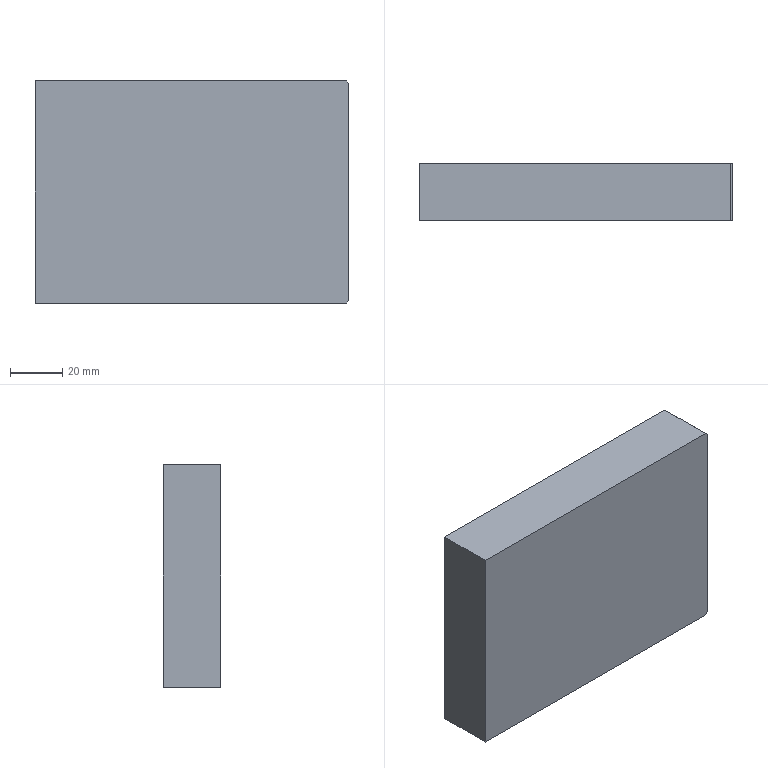Part | STEP file | B1-023 | 1 solid | 8 faces | box 120 x 22 x 85 mm | volume 224378 mm3 | plane 8
STEP:
#1=CARTESIAN_POINT('',(0.,0.,0.));
#2=DIRECTION('',(0.,0.,1.));
#3=DIRECTION('',(1.,0.,0.));
#4=AXIS2_PLACEMENT_3D('',#1,#2,#3);
#5=CARTESIAN_POINT('',(59.,11.,-42.5));
#6=VERTEX_POINT('',#5);
#7=CARTESIAN_POINT('',(-60.,11.,-42.5));
#8=VERTEX_POINT('',#7);
#9=CARTESIAN_POINT('',(60.,11.,-42.5));
#10=DIRECTION('',(-1.,0.,0.));
#11=VECTOR('',#10,1.);
#12=LINE('',#9,#11);
#13=CARTESIAN_POINT('',(60.,11.,-42.5));
#14=DIRECTION('',(0.,0.,1.));
#15=DIRECTION('',(1.,0.,0.));
#16=AXIS2_PLACEMENT_3D('',#13,#14,#15);
#17=PLANE('',#16);
#18=CARTESIAN_POINT('',(0.,0.));
#19=DIRECTION('',(-1.,0.));
#20=VECTOR('',#19,1.);
#21=LINE('',#18,#20);
#22=(GEOMETRIC_REPRESENTATION_CONTEXT(2)PARAMETRIC_REPRESENTATION_CONTEXT()REPRESENTATION_CONTEXT('',''));
#23=DEFINITIONAL_REPRESENTATION('',(#21),#22);
#24=PCURVE('',#17,#23);
#25=CARTESIAN_POINT('',(60.,11.,42.5));
#26=DIRECTION('',(0.,-1.,0.));
#27=DIRECTION('',(0.,0.,-1.));
#28=AXIS2_PLACEMENT_3D('',#25,#26,#27);
#29=PLANE('',#28);
#30=CARTESIAN_POINT('',(85.,0.));
#31=DIRECTION('',(0.,-1.));
#32=VECTOR('',#31,1.);
#33=LINE('',#30,#32);
#34=(GEOMETRIC_REPRESENTATION_CONTEXT(2)PARAMETRIC_REPRESENTATION_CONTEXT()REPRESENTATION_CONTEXT('',''));
#35=DEFINITIONAL_REPRESENTATION('',(#33),#34);
#36=PCURVE('',#29,#35);
#37=SURFACE_CURVE('',#12,(#24,#36),.PCURVE_S1.);
#38=EDGE_CURVE('',#6,#8,#37,.T.);
#39=ORIENTED_EDGE('',*,*,#38,.F.);
#40=CARTESIAN_POINT('',(59.,-11.,-42.5));
#41=VERTEX_POINT('',#40);
#42=CARTESIAN_POINT('',(59.,-11.,-42.5));
#43=DIRECTION('',(0.,-1.,0.));
#44=VECTOR('',#43,1.);
#45=LINE('',#42,#44);
#46=CARTESIAN_POINT('',(-1.,-22.));
#47=DIRECTION('',(0.,-1.));
#48=VECTOR('',#47,1.);
#49=LINE('',#46,#48);
#50=(GEOMETRIC_REPRESENTATION_CONTEXT(2)PARAMETRIC_REPRESENTATION_CONTEXT()REPRESENTATION_CONTEXT('',''));
#51=DEFINITIONAL_REPRESENTATION('',(#49),#50);
#52=PCURVE('',#17,#51);
#53=CARTESIAN_POINT('',(60.,0.,-41.5));
#54=DIRECTION('',(0.7071,0.,-0.7071));
#55=DIRECTION('',(0.,-1.,0.));
#56=AXIS2_PLACEMENT_3D('',#53,#54,#55);
#57=PLANE('',#56);
#58=CARTESIAN_POINT('',(11.,1.414));
#59=DIRECTION('',(1.,0.));
#60=VECTOR('',#59,1.);
#61=LINE('',#58,#60);
#62=(GEOMETRIC_REPRESENTATION_CONTEXT(2)PARAMETRIC_REPRESENTATION_CONTEXT()REPRESENTATION_CONTEXT('',''));
#63=DEFINITIONAL_REPRESENTATION('',(#61),#62);
#64=PCURVE('',#57,#63);
#65=SURFACE_CURVE('',#45,(#52,#64),.PCURVE_S1.);
#66=EDGE_CURVE('',#6,#41,#65,.T.);
#67=ORIENTED_EDGE('',*,*,#66,.T.);
#68=CARTESIAN_POINT('',(-60.,-11.,-42.5));
#69=VERTEX_POINT('',#68);
#70=CARTESIAN_POINT('',(60.,-11.,-42.5));
#71=DIRECTION('',(-1.,0.,0.));
#72=VECTOR('',#71,1.);
#73=LINE('',#70,#72);
#74=CARTESIAN_POINT('',(0.,-22.));
#75=DIRECTION('',(-1.,0.));
#76=VECTOR('',#75,1.);
#77=LINE('',#74,#76);
#78=(GEOMETRIC_REPRESENTATION_CONTEXT(2)PARAMETRIC_REPRESENTATION_CONTEXT()REPRESENTATION_CONTEXT('',''));
#79=DEFINITIONAL_REPRESENTATION('',(#77),#78);
#80=PCURVE('',#17,#79);
#81=CARTESIAN_POINT('',(60.,-11.,42.5));
#82=DIRECTION('',(0.,1.,0.));
#83=DIRECTION('',(0.,0.,1.));
#84=AXIS2_PLACEMENT_3D('',#81,#82,#83);
#85=PLANE('',#84);
#86=CARTESIAN_POINT('',(-85.,0.));
#87=DIRECTION('',(0.,-1.));
#88=VECTOR('',#87,1.);
#89=LINE('',#86,#88);
#90=(GEOMETRIC_REPRESENTATION_CONTEXT(2)PARAMETRIC_REPRESENTATION_CONTEXT()REPRESENTATION_CONTEXT('',''));
#91=DEFINITIONAL_REPRESENTATION('',(#89),#90);
#92=PCURVE('',#85,#91);
#93=SURFACE_CURVE('',#73,(#80,#92),.PCURVE_S1.);
#94=EDGE_CURVE('',#41,#69,#93,.T.);
#95=ORIENTED_EDGE('',*,*,#94,.T.);
#96=CARTESIAN_POINT('',(-60.,11.,-42.5));
#97=DIRECTION('',(0.,1.,0.));
#98=VECTOR('',#97,1.);
#99=LINE('',#96,#98);
#100=CARTESIAN_POINT('',(-120.,0.));
#101=DIRECTION('',(0.,1.));
#102=VECTOR('',#101,1.);
#103=LINE('',#100,#102);
#104=(GEOMETRIC_REPRESENTATION_CONTEXT(2)PARAMETRIC_REPRESENTATION_CONTEXT()REPRESENTATION_CONTEXT('',''));
#105=DEFINITIONAL_REPRESENTATION('',(#103),#104);
#106=PCURVE('',#17,#105);
#107=CARTESIAN_POINT('',(-60.,0.,0.));
#108=DIRECTION('',(1.,0.,0.));
#109=DIRECTION('',(0.,0.,-1.));
#110=AXIS2_PLACEMENT_3D('',#107,#108,#109);
#111=PLANE('',#110);
#112=CARTESIAN_POINT('',(42.5,11.));
#113=DIRECTION('',(0.,1.));
#114=VECTOR('',#113,1.);
#115=LINE('',#112,#114);
#116=(GEOMETRIC_REPRESENTATION_CONTEXT(2)PARAMETRIC_REPRESENTATION_CONTEXT()REPRESENTATION_CONTEXT('',''));
#117=DEFINITIONAL_REPRESENTATION('',(#115),#116);
#118=PCURVE('',#111,#117);
#119=SURFACE_CURVE('',#99,(#106,#118),.PCURVE_S1.);
#120=EDGE_CURVE('',#69,#8,#119,.T.);
#121=ORIENTED_EDGE('',*,*,#120,.T.);
#122=EDGE_LOOP('',(#39,#67,#95,#121));
#123=FACE_BOUND('',#122,.T.);
#124=ADVANCED_FACE('',(#123),#17,.F.);
#125=CARTESIAN_POINT('',(59.,11.,42.5));
#126=VERTEX_POINT('',#125);
#127=CARTESIAN_POINT('',(-60.,11.,42.5));
#128=VERTEX_POINT('',#127);
#129=CARTESIAN_POINT('',(60.,11.,42.5));
#130=DIRECTION('',(-1.,0.,0.));
#131=VECTOR('',#130,1.);
#132=LINE('',#129,#131);
#133=CARTESIAN_POINT('',(0.,0.));
#134=DIRECTION('',(0.,-1.));
#135=VECTOR('',#134,1.);
#136=LINE('',#133,#135);
#137=(GEOMETRIC_REPRESENTATION_CONTEXT(2)PARAMETRIC_REPRESENTATION_CONTEXT()REPRESENTATION_CONTEXT('',''));
#138=DEFINITIONAL_REPRESENTATION('',(#136),#137);
#139=PCURVE('',#29,#138);
#140=CARTESIAN_POINT('',(60.,11.,42.5));
#141=DIRECTION('',(0.,0.,-1.));
#142=DIRECTION('',(-1.,0.,0.));
#143=AXIS2_PLACEMENT_3D('',#140,#141,#142);
#144=PLANE('',#143);
#145=CARTESIAN_POINT('',(0.,0.));
#146=DIRECTION('',(1.,0.));
#147=VECTOR('',#146,1.);
#148=LINE('',#145,#147);
#149=(GEOMETRIC_REPRESENTATION_CONTEXT(2)PARAMETRIC_REPRESENTATION_CONTEXT()REPRESENTATION_CONTEXT('',''));
#150=DEFINITIONAL_REPRESENTATION('',(#148),#149);
#151=PCURVE('',#144,#150);
#152=SURFACE_CURVE('',#132,(#139,#151),.PCURVE_S1.);
#153=EDGE_CURVE('',#126,#128,#152,.T.);
#154=ORIENTED_EDGE('',*,*,#153,.F.);
#155=CARTESIAN_POINT('',(60.,11.,41.5));
#156=VERTEX_POINT('',#155);
#157=CARTESIAN_POINT('',(60.,11.,41.5));
#158=DIRECTION('',(0.7071,0.,-0.7071));
#159=VECTOR('',#158,1.);
#160=LINE('',#157,#159);
#161=CARTESIAN_POINT('',(1.,0.));
#162=DIRECTION('',(0.7071,0.7071));
#163=VECTOR('',#162,1.);
#164=LINE('',#161,#163);
#165=(GEOMETRIC_REPRESENTATION_CONTEXT(2)PARAMETRIC_REPRESENTATION_CONTEXT()REPRESENTATION_CONTEXT('',''));
#166=DEFINITIONAL_REPRESENTATION('',(#164),#165);
#167=PCURVE('',#29,#166);
#168=CARTESIAN_POINT('',(60.,0.,41.5));
#169=DIRECTION('',(0.7071,0.,0.7071));
#170=DIRECTION('',(0.,1.,0.));
#171=AXIS2_PLACEMENT_3D('',#168,#169,#170);
#172=PLANE('',#171);
#173=CARTESIAN_POINT('',(11.,0.));
#174=DIRECTION('',(0.,-1.));
#175=VECTOR('',#174,1.);
#176=LINE('',#173,#175);
#177=(GEOMETRIC_REPRESENTATION_CONTEXT(2)PARAMETRIC_REPRESENTATION_CONTEXT()REPRESENTATION_CONTEXT('',''));
#178=DEFINITIONAL_REPRESENTATION('',(#176),#177);
#179=PCURVE('',#172,#178);
#180=SURFACE_CURVE('',#160,(#167,#179),.PCURVE_S1.);
#181=EDGE_CURVE('',#126,#156,#180,.T.);
#182=ORIENTED_EDGE('',*,*,#181,.T.);
#183=CARTESIAN_POINT('',(60.,11.,-41.5));
#184=VERTEX_POINT('',#183);
#185=CARTESIAN_POINT('',(60.,11.,42.5));
#186=DIRECTION('',(0.,0.,1.));
#187=VECTOR('',#186,1.);
#188=LINE('',#185,#187);
#189=CARTESIAN_POINT('',(0.,0.));
#190=DIRECTION('',(-1.,0.));
#191=VECTOR('',#190,1.);
#192=LINE('',#189,#191);
#193=(GEOMETRIC_REPRESENTATION_CONTEXT(2)PARAMETRIC_REPRESENTATION_CONTEXT()REPRESENTATION_CONTEXT('',''));
#194=DEFINITIONAL_REPRESENTATION('',(#192),#193);
#195=PCURVE('',#29,#194);
#196=CARTESIAN_POINT('',(60.,0.,0.));
#197=DIRECTION('',(1.,0.,0.));
#198=DIRECTION('',(0.,0.,-1.));
#199=AXIS2_PLACEMENT_3D('',#196,#197,#198);
#200=PLANE('',#199);
#201=CARTESIAN_POINT('',(-42.5,11.));
#202=DIRECTION('',(-1.,0.));
#203=VECTOR('',#202,1.);
#204=LINE('',#201,#203);
#205=(GEOMETRIC_REPRESENTATION_CONTEXT(2)PARAMETRIC_REPRESENTATION_CONTEXT()REPRESENTATION_CONTEXT('',''));
#206=DEFINITIONAL_REPRESENTATION('',(#204),#205);
#207=PCURVE('',#200,#206);
#208=SURFACE_CURVE('',#188,(#195,#207),.PCURVE_S1.);
#209=EDGE_CURVE('',#184,#156,#208,.T.);
#210=ORIENTED_EDGE('',*,*,#209,.F.);
#211=CARTESIAN_POINT('',(60.,11.,-41.5));
#212=DIRECTION('',(-0.7071,0.,-0.7071));
#213=VECTOR('',#212,1.);
#214=LINE('',#211,#213);
#215=CARTESIAN_POINT('',(84.,0.));
#216=DIRECTION('',(0.7071,-0.7071));
#217=VECTOR('',#216,1.);
#218=LINE('',#215,#217);
#219=(GEOMETRIC_REPRESENTATION_CONTEXT(2)PARAMETRIC_REPRESENTATION_CONTEXT()REPRESENTATION_CONTEXT('',''));
#220=DEFINITIONAL_REPRESENTATION('',(#218),#219);
#221=PCURVE('',#29,#220);
#222=CARTESIAN_POINT('',(-11.,0.));
#223=DIRECTION('',(0.,1.));
#224=VECTOR('',#223,1.);
#225=LINE('',#222,#224);
#226=(GEOMETRIC_REPRESENTATION_CONTEXT(2)PARAMETRIC_REPRESENTATION_CONTEXT()REPRESENTATION_CONTEXT('',''));
#227=DEFINITIONAL_REPRESENTATION('',(#225),#226);
#228=PCURVE('',#57,#227);
#229=SURFACE_CURVE('',#214,(#221,#228),.PCURVE_S1.);
#230=EDGE_CURVE('',#184,#6,#229,.T.);
#231=ORIENTED_EDGE('',*,*,#230,.T.);
#232=ORIENTED_EDGE('',*,*,#38,.T.);
#233=CARTESIAN_POINT('',(-60.,11.,42.5));
#234=DIRECTION('',(0.,0.,1.));
#235=VECTOR('',#234,1.);
#236=LINE('',#233,#235);
#237=CARTESIAN_POINT('',(0.,-120.));
#238=DIRECTION('',(-1.,0.));
#239=VECTOR('',#238,1.);
#240=LINE('',#237,#239);
#241=(GEOMETRIC_REPRESENTATION_CONTEXT(2)PARAMETRIC_REPRESENTATION_CONTEXT()REPRESENTATION_CONTEXT('',''));
#242=DEFINITIONAL_REPRESENTATION('',(#240),#241);
#243=PCURVE('',#29,#242);
#244=CARTESIAN_POINT('',(-42.5,11.));
#245=DIRECTION('',(-1.,0.));
#246=VECTOR('',#245,1.);
#247=LINE('',#244,#246);
#248=(GEOMETRIC_REPRESENTATION_CONTEXT(2)PARAMETRIC_REPRESENTATION_CONTEXT()REPRESENTATION_CONTEXT('',''));
#249=DEFINITIONAL_REPRESENTATION('',(#247),#248);
#250=PCURVE('',#111,#249);
#251=SURFACE_CURVE('',#236,(#243,#250),.PCURVE_S1.);
#252=EDGE_CURVE('',#8,#128,#251,.T.);
#253=ORIENTED_EDGE('',*,*,#252,.T.);
#254=EDGE_LOOP('',(#154,#182,#210,#231,#232,#253));
#255=FACE_BOUND('',#254,.T.);
#256=ADVANCED_FACE('',(#255),#29,.F.);
#257=CARTESIAN_POINT('',(59.,-11.,42.5));
#258=VERTEX_POINT('',#257);
#259=CARTESIAN_POINT('',(-60.,-11.,42.5));
#260=VERTEX_POINT('',#259);
#261=CARTESIAN_POINT('',(60.,-11.,42.5));
#262=DIRECTION('',(-1.,0.,0.));
#263=VECTOR('',#262,1.);
#264=LINE('',#261,#263);
#265=CARTESIAN_POINT('',(0.,-22.));
#266=DIRECTION('',(1.,0.));
#267=VECTOR('',#266,1.);
#268=LINE('',#265,#267);
#269=(GEOMETRIC_REPRESENTATION_CONTEXT(2)PARAMETRIC_REPRESENTATION_CONTEXT()REPRESENTATION_CONTEXT('',''));
#270=DEFINITIONAL_REPRESENTATION('',(#268),#269);
#271=PCURVE('',#144,#270);
#272=CARTESIAN_POINT('',(0.,0.));
#273=DIRECTION('',(0.,-1.));
#274=VECTOR('',#273,1.);
#275=LINE('',#272,#274);
#276=(GEOMETRIC_REPRESENTATION_CONTEXT(2)PARAMETRIC_REPRESENTATION_CONTEXT()REPRESENTATION_CONTEXT('',''));
#277=DEFINITIONAL_REPRESENTATION('',(#275),#276);
#278=PCURVE('',#85,#277);
#279=SURFACE_CURVE('',#264,(#271,#278),.PCURVE_S1.);
#280=EDGE_CURVE('',#258,#260,#279,.T.);
#281=ORIENTED_EDGE('',*,*,#280,.F.);
#282=CARTESIAN_POINT('',(59.,11.,42.5));
#283=DIRECTION('',(0.,1.,0.));
#284=VECTOR('',#283,1.);
#285=LINE('',#282,#284);
#286=CARTESIAN_POINT('',(1.,0.));
#287=DIRECTION('',(0.,1.));
#288=VECTOR('',#287,1.);
#289=LINE('',#286,#288);
#290=(GEOMETRIC_REPRESENTATION_CONTEXT(2)PARAMETRIC_REPRESENTATION_CONTEXT()REPRESENTATION_CONTEXT('',''));
#291=DEFINITIONAL_REPRESENTATION('',(#289),#290);
#292=PCURVE('',#144,#291);
#293=CARTESIAN_POINT('',(11.,1.414));
#294=DIRECTION('',(1.,0.));
#295=VECTOR('',#294,1.);
#296=LINE('',#293,#295);
#297=(GEOMETRIC_REPRESENTATION_CONTEXT(2)PARAMETRIC_REPRESENTATION_CONTEXT()REPRESENTATION_CONTEXT('',''));
#298=DEFINITIONAL_REPRESENTATION('',(#296),#297);
#299=PCURVE('',#172,#298);
#300=SURFACE_CURVE('',#285,(#292,#299),.PCURVE_S1.);
#301=EDGE_CURVE('',#258,#126,#300,.T.);
#302=ORIENTED_EDGE('',*,*,#301,.T.);
#303=ORIENTED_EDGE('',*,*,#153,.T.);
#304=CARTESIAN_POINT('',(-60.,11.,42.5));
#305=DIRECTION('',(0.,-1.,0.));
#306=VECTOR('',#305,1.);
#307=LINE('',#304,#306);
#308=CARTESIAN_POINT('',(120.,0.));
#309=DIRECTION('',(0.,-1.));
#310=VECTOR('',#309,1.);
#311=LINE('',#308,#310);
#312=(GEOMETRIC_REPRESENTATION_CONTEXT(2)PARAMETRIC_REPRESENTATION_CONTEXT()REPRESENTATION_CONTEXT('',''));
#313=DEFINITIONAL_REPRESENTATION('',(#311),#312);
#314=PCURVE('',#144,#313);
#315=CARTESIAN_POINT('',(-42.5,11.));
#316=DIRECTION('',(0.,-1.));
#317=VECTOR('',#316,1.);
#318=LINE('',#315,#317);
#319=(GEOMETRIC_REPRESENTATION_CONTEXT(2)PARAMETRIC_REPRESENTATION_CONTEXT()REPRESENTATION_CONTEXT('',''));
#320=DEFINITIONAL_REPRESENTATION('',(#318),#319);
#321=PCURVE('',#111,#320);
#322=SURFACE_CURVE('',#307,(#314,#321),.PCURVE_S1.);
#323=EDGE_CURVE('',#128,#260,#322,.T.);
#324=ORIENTED_EDGE('',*,*,#323,.T.);
#325=EDGE_LOOP('',(#281,#302,#303,#324));
#326=FACE_BOUND('',#325,.T.);
#327=ADVANCED_FACE('',(#326),#144,.F.);
#328=CARTESIAN_POINT('',(60.,-11.,41.5));
#329=VERTEX_POINT('',#328);
#330=CARTESIAN_POINT('',(60.,-11.,-41.5));
#331=VERTEX_POINT('',#330);
#332=CARTESIAN_POINT('',(60.,-11.,42.5));
#333=DIRECTION('',(0.,0.,-1.));
#334=VECTOR('',#333,1.);
#335=LINE('',#332,#334);
#336=CARTESIAN_POINT('',(0.,0.));
#337=DIRECTION('',(-1.,0.));
#338=VECTOR('',#337,1.);
#339=LINE('',#336,#338);
#340=(GEOMETRIC_REPRESENTATION_CONTEXT(2)PARAMETRIC_REPRESENTATION_CONTEXT()REPRESENTATION_CONTEXT('',''));
#341=DEFINITIONAL_REPRESENTATION('',(#339),#340);
#342=PCURVE('',#85,#341);
#343=CARTESIAN_POINT('',(-42.5,-11.));
#344=DIRECTION('',(1.,0.));
#345=VECTOR('',#344,1.);
#346=LINE('',#343,#345);
#347=(GEOMETRIC_REPRESENTATION_CONTEXT(2)PARAMETRIC_REPRESENTATION_CONTEXT()REPRESENTATION_CONTEXT('',''));
#348=DEFINITIONAL_REPRESENTATION('',(#346),#347);
#349=PCURVE('',#200,#348);
#350=SURFACE_CURVE('',#335,(#342,#349),.PCURVE_S1.);
#351=EDGE_CURVE('',#329,#331,#350,.T.);
#352=ORIENTED_EDGE('',*,*,#351,.F.);
#353=CARTESIAN_POINT('',(60.,-11.,41.5));
#354=DIRECTION('',(-0.7071,0.,0.7071));
#355=VECTOR('',#354,1.);
#356=LINE('',#353,#355);
#357=CARTESIAN_POINT('',(-1.,0.));
#358=DIRECTION('',(0.7071,-0.7071));
#359=VECTOR('',#358,1.);
#360=LINE('',#357,#359);
#361=(GEOMETRIC_REPRESENTATION_CONTEXT(2)PARAMETRIC_REPRESENTATION_CONTEXT()REPRESENTATION_CONTEXT('',''));
#362=DEFINITIONAL_REPRESENTATION('',(#360),#361);
#363=PCURVE('',#85,#362);
#364=CARTESIAN_POINT('',(-11.,0.));
#365=DIRECTION('',(0.,1.));
#366=VECTOR('',#365,1.);
#367=LINE('',#364,#366);
#368=(GEOMETRIC_REPRESENTATION_CONTEXT(2)PARAMETRIC_REPRESENTATION_CONTEXT()REPRESENTATION_CONTEXT('',''));
#369=DEFINITIONAL_REPRESENTATION('',(#367),#368);
#370=PCURVE('',#172,#369);
#371=SURFACE_CURVE('',#356,(#363,#370),.PCURVE_S1.);
#372=EDGE_CURVE('',#329,#258,#371,.T.);
#373=ORIENTED_EDGE('',*,*,#372,.T.);
#374=ORIENTED_EDGE('',*,*,#280,.T.);
#375=CARTESIAN_POINT('',(-60.,-11.,42.5));
#376=DIRECTION('',(0.,0.,-1.));
#377=VECTOR('',#376,1.);
#378=LINE('',#375,#377);
#379=CARTESIAN_POINT('',(0.,-120.));
#380=DIRECTION('',(-1.,0.));
#381=VECTOR('',#380,1.);
#382=LINE('',#379,#381);
#383=(GEOMETRIC_REPRESENTATION_CONTEXT(2)PARAMETRIC_REPRESENTATION_CONTEXT()REPRESENTATION_CONTEXT('',''));
#384=DEFINITIONAL_REPRESENTATION('',(#382),#383);
#385=PCURVE('',#85,#384);
#386=CARTESIAN_POINT('',(-42.5,-11.));
#387=DIRECTION('',(1.,0.));
#388=VECTOR('',#387,1.);
#389=LINE('',#386,#388);
#390=(GEOMETRIC_REPRESENTATION_CONTEXT(2)PARAMETRIC_REPRESENTATION_CONTEXT()REPRESENTATION_CONTEXT('',''));
#391=DEFINITIONAL_REPRESENTATION('',(#389),#390);
#392=PCURVE('',#111,#391);
#393=SURFACE_CURVE('',#378,(#385,#392),.PCURVE_S1.);
#394=EDGE_CURVE('',#260,#69,#393,.T.);
#395=ORIENTED_EDGE('',*,*,#394,.T.);
#396=ORIENTED_EDGE('',*,*,#94,.F.);
#397=CARTESIAN_POINT('',(60.,-11.,-41.5));
#398=DIRECTION('',(0.7071,0.,0.7071));
#399=VECTOR('',#398,1.);
#400=LINE('',#397,#399);
#401=CARTESIAN_POINT('',(-84.,0.));
#402=DIRECTION('',(0.7071,0.7071));
#403=VECTOR('',#402,1.);
#404=LINE('',#401,#403);
#405=(GEOMETRIC_REPRESENTATION_CONTEXT(2)PARAMETRIC_REPRESENTATION_CONTEXT()REPRESENTATION_CONTEXT('',''));
#406=DEFINITIONAL_REPRESENTATION('',(#404),#405);
#407=PCURVE('',#85,#406);
#408=CARTESIAN_POINT('',(11.,0.));
#409=DIRECTION('',(0.,-1.));
#410=VECTOR('',#409,1.);
#411=LINE('',#408,#410);
#412=(GEOMETRIC_REPRESENTATION_CONTEXT(2)PARAMETRIC_REPRESENTATION_CONTEXT()REPRESENTATION_CONTEXT('',''));
#413=DEFINITIONAL_REPRESENTATION('',(#411),#412);
#414=PCURVE('',#57,#413);
#415=SURFACE_CURVE('',#400,(#407,#414),.PCURVE_S1.);
#416=EDGE_CURVE('',#41,#331,#415,.T.);
#417=ORIENTED_EDGE('',*,*,#416,.T.);
#418=EDGE_LOOP('',(#352,#373,#374,#395,#396,#417));
#419=FACE_BOUND('',#418,.T.);
#420=ADVANCED_FACE('',(#419),#85,.F.);
#421=ORIENTED_EDGE('',*,*,#209,.T.);
#422=CARTESIAN_POINT('',(60.,-11.,41.5));
#423=DIRECTION('',(0.,-1.,0.));
#424=VECTOR('',#423,1.);
#425=LINE('',#422,#424);
#426=CARTESIAN_POINT('',(-41.5,-11.));
#427=DIRECTION('',(0.,-1.));
#428=VECTOR('',#427,1.);
#429=LINE('',#426,#428);
#430=(GEOMETRIC_REPRESENTATION_CONTEXT(2)PARAMETRIC_REPRESENTATION_CONTEXT()REPRESENTATION_CONTEXT('',''));
#431=DEFINITIONAL_REPRESENTATION('',(#429),#430);
#432=PCURVE('',#200,#431);
#433=CARTESIAN_POINT('',(-11.,0.));
#434=DIRECTION('',(-1.,0.));
#435=VECTOR('',#434,1.);
#436=LINE('',#433,#435);
#437=(GEOMETRIC_REPRESENTATION_CONTEXT(2)PARAMETRIC_REPRESENTATION_CONTEXT()REPRESENTATION_CONTEXT('',''));
#438=DEFINITIONAL_REPRESENTATION('',(#436),#437);
#439=PCURVE('',#172,#438);
#440=SURFACE_CURVE('',#425,(#432,#439),.PCURVE_S1.);
#441=EDGE_CURVE('',#156,#329,#440,.T.);
#442=ORIENTED_EDGE('',*,*,#441,.T.);
#443=ORIENTED_EDGE('',*,*,#351,.T.);
#444=CARTESIAN_POINT('',(60.,11.,-41.5));
#445=DIRECTION('',(0.,1.,0.));
#446=VECTOR('',#445,1.);
#447=LINE('',#444,#446);
#448=CARTESIAN_POINT('',(41.5,11.));
#449=DIRECTION('',(0.,1.));
#450=VECTOR('',#449,1.);
#451=LINE('',#448,#450);
#452=(GEOMETRIC_REPRESENTATION_CONTEXT(2)PARAMETRIC_REPRESENTATION_CONTEXT()REPRESENTATION_CONTEXT('',''));
#453=DEFINITIONAL_REPRESENTATION('',(#451),#452);
#454=PCURVE('',#200,#453);
#455=CARTESIAN_POINT('',(-11.,0.));
#456=DIRECTION('',(-1.,0.));
#457=VECTOR('',#456,1.);
#458=LINE('',#455,#457);
#459=(GEOMETRIC_REPRESENTATION_CONTEXT(2)PARAMETRIC_REPRESENTATION_CONTEXT()REPRESENTATION_CONTEXT('',''));
#460=DEFINITIONAL_REPRESENTATION('',(#458),#459);
#461=PCURVE('',#57,#460);
#462=SURFACE_CURVE('',#447,(#454,#461),.PCURVE_S1.);
#463=EDGE_CURVE('',#331,#184,#462,.T.);
#464=ORIENTED_EDGE('',*,*,#463,.T.);
#465=EDGE_LOOP('',(#421,#442,#443,#464));
#466=FACE_BOUND('',#465,.T.);
#467=ADVANCED_FACE('',(#466),#200,.T.);
#468=ORIENTED_EDGE('',*,*,#120,.F.);
#469=ORIENTED_EDGE('',*,*,#394,.F.);
#470=ORIENTED_EDGE('',*,*,#323,.F.);
#471=ORIENTED_EDGE('',*,*,#252,.F.);
#472=EDGE_LOOP('',(#468,#469,#470,#471));
#473=FACE_BOUND('',#472,.T.);
#474=ADVANCED_FACE('',(#473),#111,.F.);
#475=ORIENTED_EDGE('',*,*,#181,.F.);
#476=ORIENTED_EDGE('',*,*,#301,.F.);
#477=ORIENTED_EDGE('',*,*,#372,.F.);
#478=ORIENTED_EDGE('',*,*,#441,.F.);
#479=EDGE_LOOP('',(#475,#476,#477,#478));
#480=FACE_BOUND('',#479,.T.);
#481=ADVANCED_FACE('',(#480),#172,.T.);
#482=ORIENTED_EDGE('',*,*,#416,.F.);
#483=ORIENTED_EDGE('',*,*,#66,.F.);
#484=ORIENTED_EDGE('',*,*,#230,.F.);
#485=ORIENTED_EDGE('',*,*,#463,.F.);
#486=EDGE_LOOP('',(#482,#483,#484,#485));
#487=FACE_BOUND('',#486,.T.);
#488=ADVANCED_FACE('',(#487),#57,.T.);
#489=CLOSED_SHELL('',(#124,#256,#327,#420,#467,#474,#481,#488));
#490=MANIFOLD_SOLID_BREP('',#489);
#491=(LENGTH_UNIT()NAMED_UNIT(*)SI_UNIT(.MILLI.,.METRE.));
#492=UNCERTAINTY_MEASURE_WITH_UNIT(LENGTH_MEASURE(0.0000001),#491,'','');
#493=(NAMED_UNIT(*)PLANE_ANGLE_UNIT()SI_UNIT($,.RADIAN.));
#494=(NAMED_UNIT(*)SI_UNIT($,.STERADIAN.)SOLID_ANGLE_UNIT());
#495=(GEOMETRIC_REPRESENTATION_CONTEXT(3)GLOBAL_UNCERTAINTY_ASSIGNED_CONTEXT((#492))GLOBAL_UNIT_ASSIGNED_CONTEXT((#491,#493,#494))REPRESENTATION_CONTEXT('',''));
#496=ADVANCED_BREP_SHAPE_REPRESENTATION('',(#4,#490),#495);